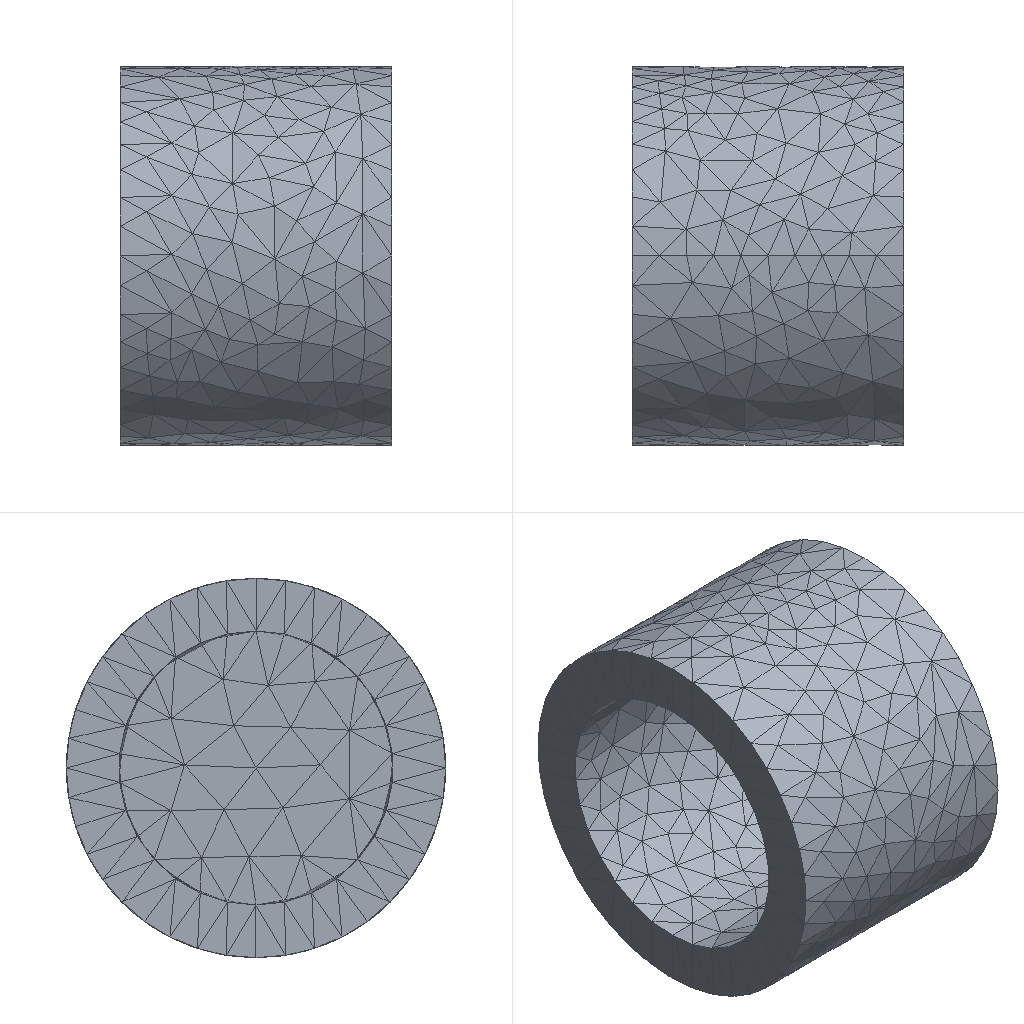Simulation study | ansys workbench
Ansys APDL input file, long lists of numbers shortened:
/batch
/config,noeldb,1     ! force off writing results to database
*get,_wallstrt,active,,time,wall
! ANSYS input file written by Workbench version 2022 R1
! File used for geometry attach:
/title,wbnew--____ (A5)
! ****** Begin Custom Load Command Snippet ******
/COM, ACT Extensions:
/COM,     LSDYNA, 2021.1
/COM,
! ****** End   Custom Load Command Snippet ******
*DIM,_wb_ProjectScratch_dir,string,248
_wb_ProjectScratch_dir(1) = ''
*DIM,_wb_SolverFiles_dir,string,248
_wb_SolverFiles_dir(1) = ''
*DIM,_wb_userfiles_dir,string,248
_wb_userfiles_dir(1) = ''
/com,--- Data in consistent NMM units. See Solving Units in the help system for more information.
/units,MPA
/nopr
/wb,file,start              !  signify a WB generated input file
/prep7
! Turn off shape checking because checks already performed inside WB mesher.
! See help system for more information.
SHPP,OFF,,NOWARN
/nolist
etcon,set             ! allow ANSYS to choose best KEYOP's for 180x elements, resets any applicable keyopt to MAPDL defaults
/com,*********** Nodes for the whole assembly ***********
nblock,3,,5033
(1i9,3e20.9e3)
        1     1.299000000E+03     0.000000000E+00     1.443258926E+02
! (4575 more lines like these left out)
-1
/wb,elem,start            !  set before creation of elements
/com,*********** Elements for Body 1 "__1-FreeParts|__-__3" ***********
et,1,187
eblock,19,solid,,2524
(19i9)
        1        1        1        1        0        0        0        0       10        0        1      597      650      736      677     4278     4479     4282     4279
! (5047 more lines like these left out)
-1
/wb,elem,end               !  done creating elements
/com,*********** Send User Defined Coordinate System(s) ***********
csys,0
toffst,273.15,  ! Temperature offset from absolute zero
/com,*********** Set Reference Temperature ***********
tref,22.
/wb,mat,start              !  starting to send materials
/com,*********** Send Materials ***********
Temperature = 'TEMP' ! Temperature
MP,DENS,1,7.85e-09,	! tonne mm^-3
MP,ALPX,1,1.2e-05,	! C^-1
MP,C,1,434000000,	! mm^2 s^-2 C^-1
MP,KXX,1,60.5,	! tonne mm s^-3 C^-1
MP,RSVX,1,0.00017,	! ohm mm
MP,EX,1,200000,	! tonne s^-2 mm^-1
MP,NUXY,1,0.3,
MP,MURX,1,10000,
/wb,mat,end                !  done sending materials
!************************* Model Summary ********************
!__1-FreeParts|__-__3,	结构钢,	matid,	1
!************************* End Model Summary ********************
! get the diagonal of the bounding box. Needed later for other things
*get,_xmin,node,,mnloc,x
*get,_ymin,node,,mnloc,y
*get,_zmin,node,,mnloc,z
*get,_xmax,node,,mxloc,x
*get,_ymax,node,,mxloc,y
*get,_zmax,node,,mxloc,z
_ASMDIAG=(_xmax-_xmin)*(_xmax-_xmin)+(_ymax-_ymin)*(_ymax-_ymin)+(_zmax-_zmin)*(_zmax-_zmin)
_ASMDIAG=SQRT(_ASMDIAG)
/wb,contact,start          !  starting to send contact
/wb,contact,end            !  done creating contacts
/golist
/wb,load,start             !  starting to send loads
/com,*********** Fixed Supports ***********
CMBLOCK,_FIXEDSU,NODE,      245
(8i10)
         1         2         3         4         5         6         7         8
! (30 more lines like these left out)
cmsel,s,_FIXEDSU
d,all,all
nsel,all
/com,*********** Define Pressure Using Surface Effect Elements "__" ***********
et,2,154
eblock,10,,,588
(15i9)
     3687        2        2        2        0       23        2      152      152      744      745      152      857
! (587 more lines like these left out)
-1
esel,s,type,,2
keyop,2,7,0                ! Use deformed area for application of load
esel,all
/com,*********** Define Pressure Using Surface Effect Elements "__ 2" ***********
et,3,154
eblock,10,,,340
(15i9)
     4275        3        3        3        0      296      117      313      313     1568     1569      313     2562
! (339 more lines like these left out)
-1
esel,s,type,,3
keyop,3,7,0                ! Use deformed area for application of load
esel,all
esel,all
/gst,on,on
fini
*get,_numnode,node,0,count
*get,_numelem,elem,0,count
*get, _MAXELEMNUM, elem, 0, NUM, MAX
*get, _MAXNODENUM, node, 0, NUM, MAX
*get, _MAXELEMTYPE, etyp, 0, NUM, MAX
*get, _MAXREALCONST, real, 0, NUM, MAX
/go
/wb,load,end               !  done creating loads
/com,--- Number of total nodes = %_numnode%
/com,--- Number of contact elements = 928
/com,--- Number of spring elements = 0
/com,--- Number of bearing elements = 0
/com,--- Number of solid elements = 2524
/com,--- Number of condensed parts = 0
/com,--- Number of total elements = %_numelem%
*get,_wallbsol,active,,time,wall
/com,****************************************************************************
/com,*************************    SOLUTION       ********************************
/com,****************************************************************************
/solu
antype,0                   ! static analysis
_thickRatio=  0     ! Ratio of thick parts in the model
eqsl,sparse,,,,,1
cntr,print,1               ! print out contact info and also make no initial contact an error
dmpoption,emat,no             ! Don't combine emat file for DANSYS
dmpoption,esav,no             ! Don't combine esav file for DANSYS
nldiag,cont,iter           ! print out contact info each equilibrium iteration
rescontrol,,none                 ! Do not keep any restart files
/com,****************************************************
/com,******************* SOLVE FOR LS 1 OF 1 ****************
esel,s,type,,2
nsle
sf,all,pres,20.
esel,s,type,,3
nsle
sf,all,pres,60.
nsel,all
esel,all
esel,all
/nopr
/gopr
nsub,1,1,1
time,1.
outres,erase
outres,all,none
outres,nsol,all,
outres,rsol,all
outres,eangl,all
outres,etmp,all
outres,veng,all
outres,strs,all,
outres,epel,all,
outres,eppl,all,
outres,cont,all,
! *********** WB SOLVE COMMAND ***********
! check interactive state
*get,ANSINTER_,active,,int
*if,ANSINTER_,ne,0,then
/eof
*endif
solve
/com *************** Write FE CONNECTORS *********
CEWRITE,file,ce,,INTE
/com,****************************************************
/com,*************** FINISHED SOLVE FOR LS 1 *************
*get,_wallasol,active,,time,wall
/nopr
*get,_numnode,node,0,count
*get,_numelem,elem,0,count
*get, _MAXELEMNUM, elem, 0, NUM, MAX
*get, _MAXNODENUM, node, 0, NUM, MAX,,,INTERNAL
*get, _MAXELEMTYPE, etyp, 0, NUM, MAX
*get, _MAXREALCONST, real, 0, NUM, MAX
/gopr
/post1
xmlo,ENCODING,ISO-8859-1
xmlo,parm
/xml,parm,xml
fini
/gopr
*get,_walldone,active,,time,wall
_preptime=(_wallbsol-_wallstrt)*3600
_solvtime=(_wallasol-_wallbsol)*3600
_posttime=(_walldone-_wallasol)*3600
_totaltim=(_walldone-_wallstrt)*3600
*get,_dlbratio,active,0,solu,dlbr
*get,_combtime,active,0,solu,comb
*get,_ssmode,active,0,solu,ssmm
*get,_ndofs,active,0,solu,ndof
*get,_sol_end_time,active,0,set,time
*if,_sol_end_time,eq,1.,then
/fclean				!clean distributed files
*endif
/com,--- Total number of nodes = %_numnode%
/com,--- Total number of elements = %_numelem%
/com,--- Element load balance ratio = %_dlbratio%
/com,--- Time to combine distributed files = %_combtime%
/com,--- Sparse memory mode = %_ssmode%
/com,--- Number of DOF = %_ndofs%
/wb,file,end               ! done with WB generated input